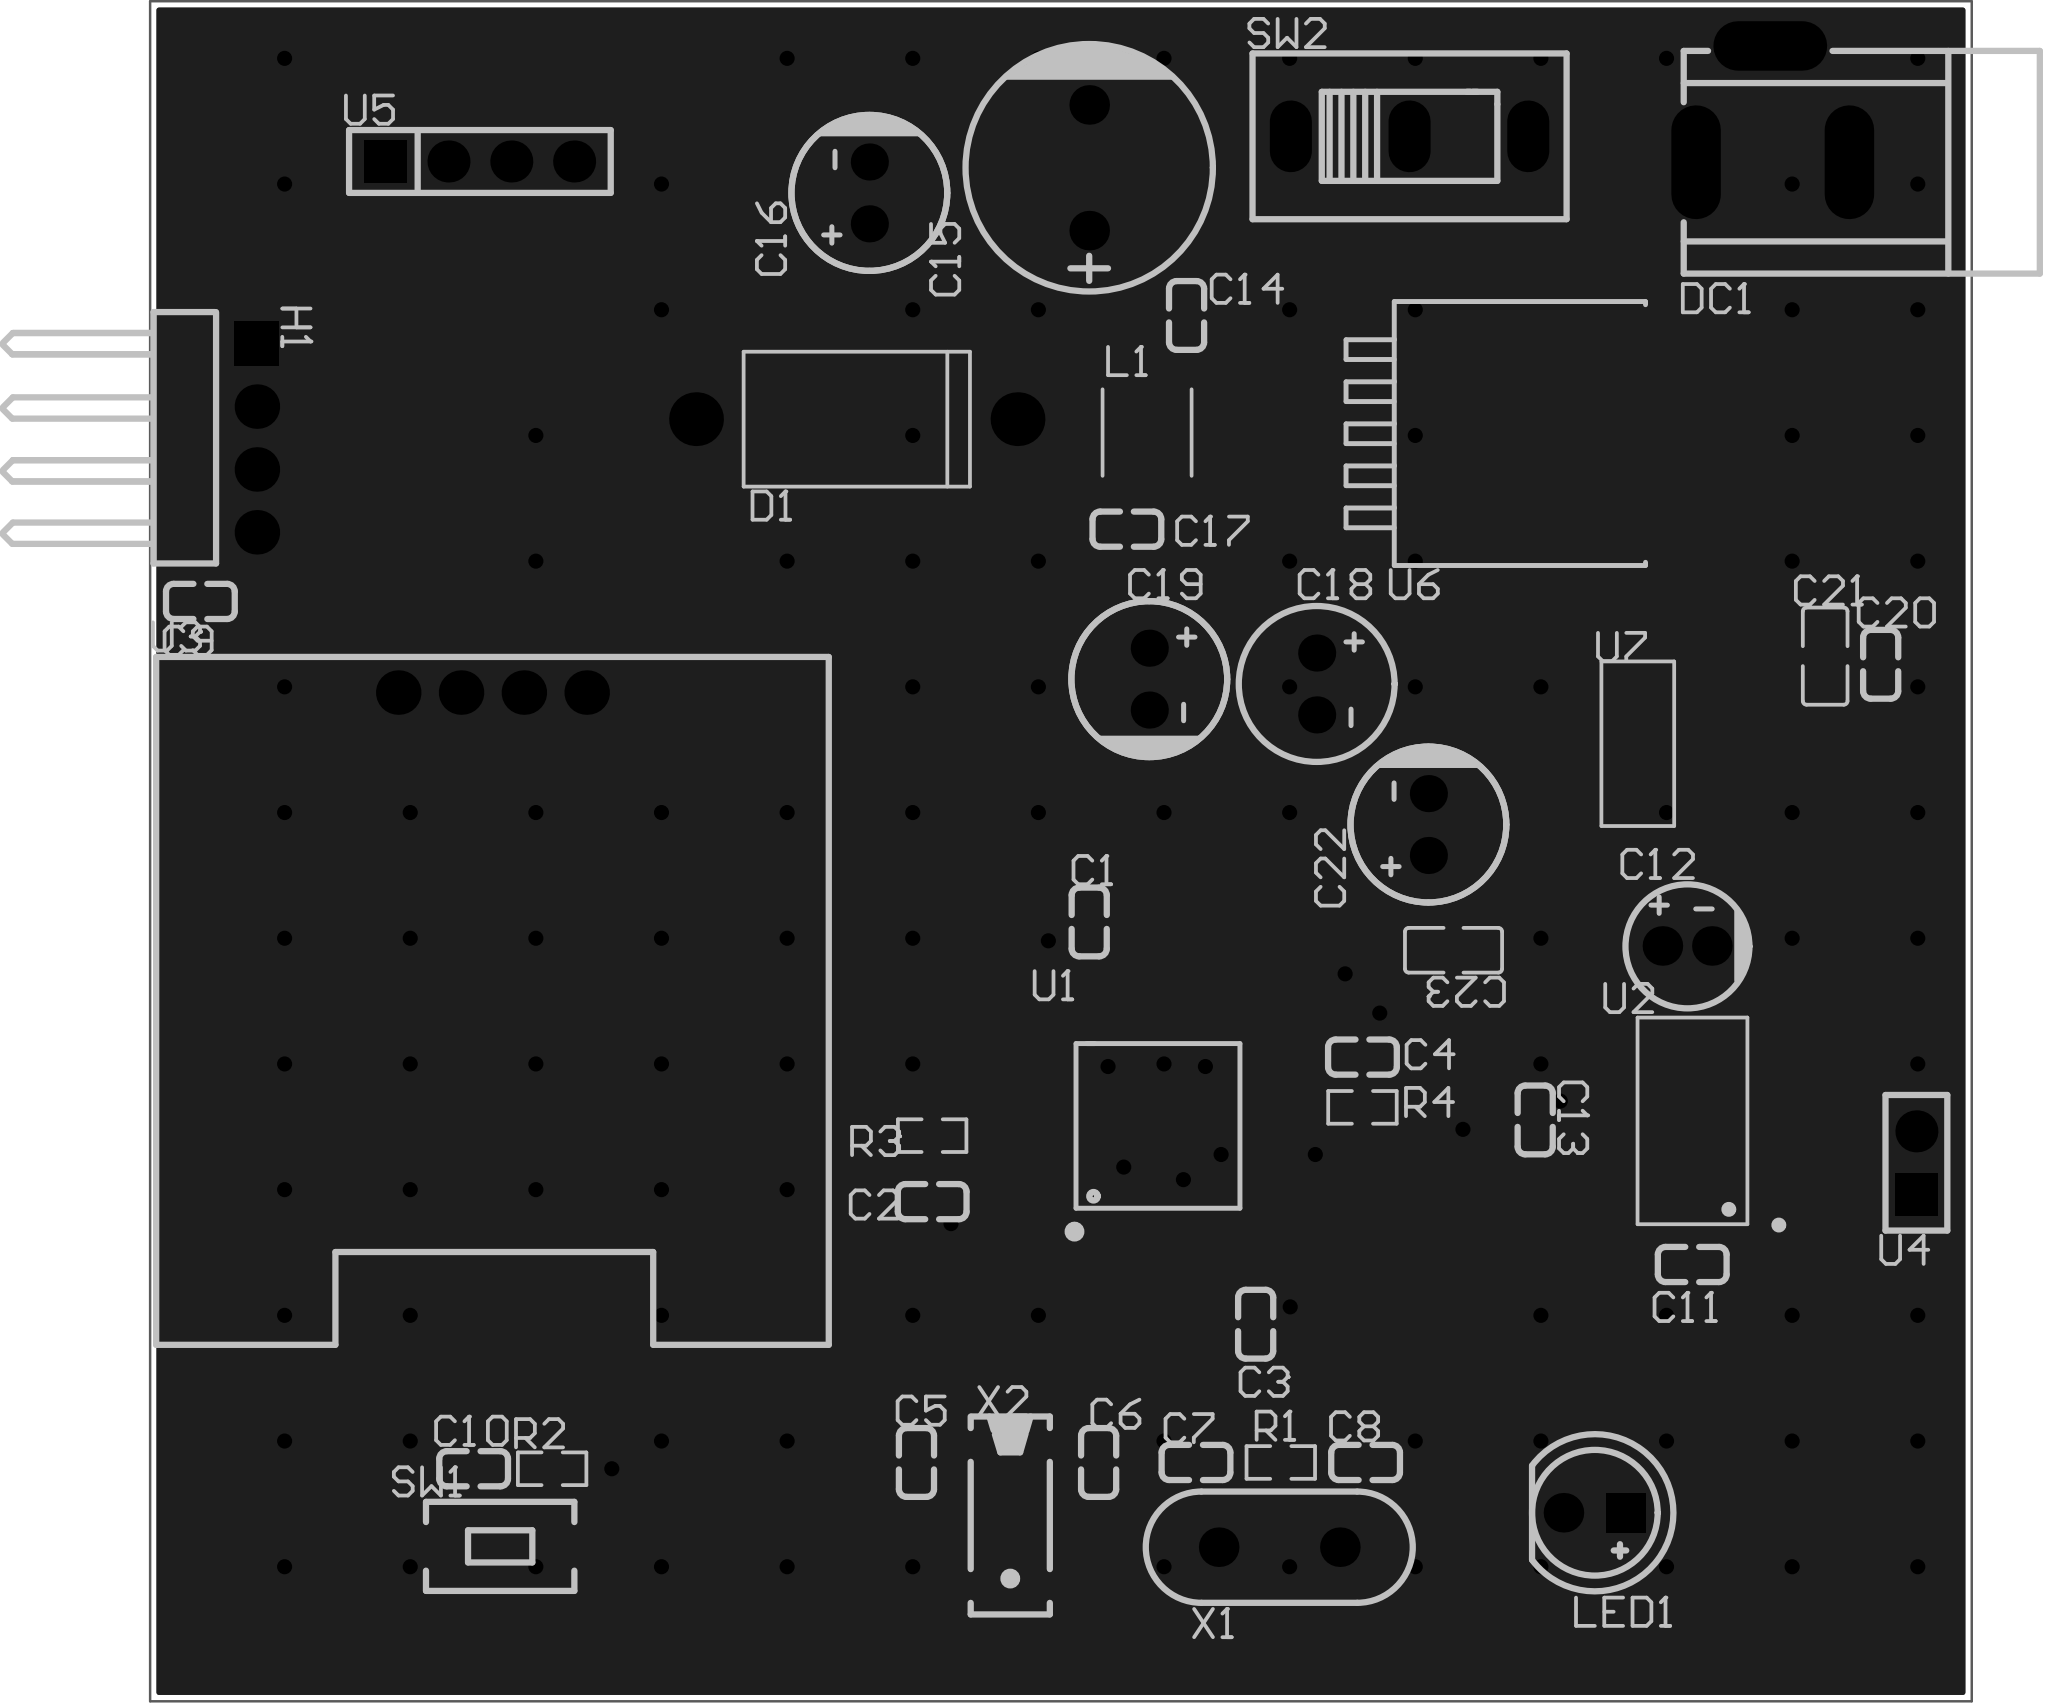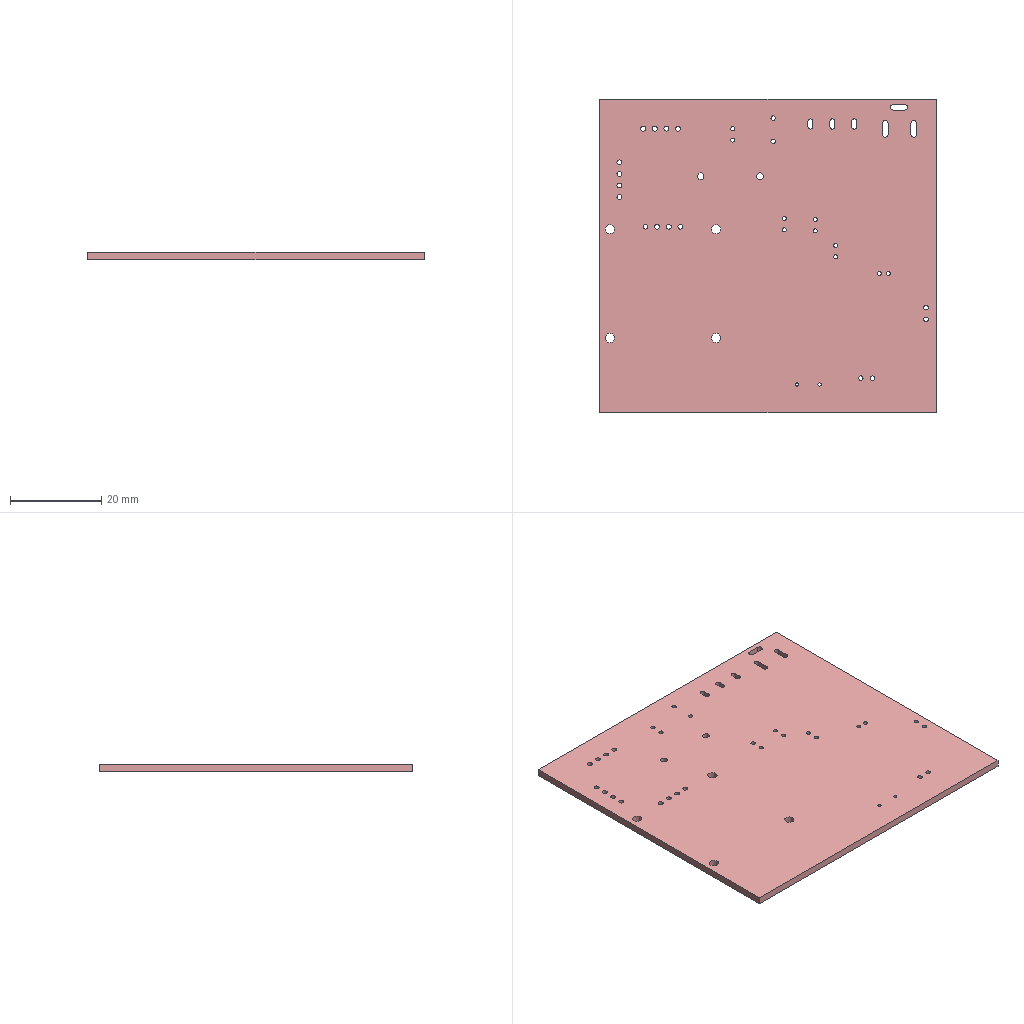Circuit board layout | Altium Designer | box 73.7 x 68.7 x 1.6 mm
Layer stack:
# Altium Designer layer stack of  (unit mm; dielectric type: 0 none, 1 core, 2 prepreg, 3 surface material)
index,name,kind,layer,copper_thickness_mm,dielectric_type,dielectric_thickness_mm,dielectric_material,dielectric_constant
0,Top Paste Mask Layer,other,,,,,,
1,Top Silkscreen Layer,other,,,,,,
2,Top Solder Mask Layer,dielectric,,,3,0.01,,3.3
3,Top Layer,copper,Top Layer,0.035,,,,
4,Dielectric1,dielectric,,,3,1.51,FR4,4.5
5,Bottom Layer,copper,Bottom Layer,0.035,,,,
6,Bottom Solder Mask Layer,dielectric,,,3,0.01,,3.3
7,Bottom Silkscreen Layer,other,,,,,,
8,Bottom Paste Mask Layer,other,,,,,,
# drill layer pairs: low layer,high layer
drill_pair,Top Layer,Bottom Layer
Part placement:
Designator,Comment,Layer,Footprint,Center-X(mm),Center-Y(mm),Rotation
C1,100nF,TopLayer,C0603,124.587,124.333,270
C2,100nF,TopLayer,C0603,118.237,113.03,0
C3,100nF,TopLayer,C0603,131.318,108.077,90
C4,100nF,TopLayer,C0603,135.636,118.872,180
C5,20pF,TopLayer,C0603,117.602,102.489,270
C6,20pF,TopLayer,C0603,124.968,102.489,270
C7,20pF,TopLayer,C0603,128.905,102.489,180
C8,20pF,TopLayer,C0603,135.763,102.489,0
C9,100nF,TopLayer,C0603,88.646,137.287,180
C10,1uF,TopLayer,C0603,99.695,102.235,0
C11,100nF,TopLayer,C0603,148.971,110.49,180
C12,10uF,TopLayer,CAP-TH_BD5.0-P2.00-D0.5-FD-A,148.765,123.364,0
C13,100nF,TopLayer,C0603,142.621,116.332,270
C14,100nF,TopLayer,C0603,128.524,148.844,270
C15,220uF,TopLayer,CAP-TH_BD10.0-P5.00-D1.0-FD,124.587,154.813,90
C16,100uF,TopLayer,CAP-TH_BD6.3-P2.50-D0.5-FD,115.697,153.797,90
C17,100nF,TopLayer,C0603,126.111,140.208,0
C18,220uF,TopLayer,CAP-TH_BD6.3-P2.50-D0.5-FD_DXW025M227E112S1AA,133.785,133.951,270
C19,100uF,TopLayer,CAP-TH_BD6.3-P2.50-D0.5-FD,127.016,134.147,270
C20,100nF,TopLayer,C0603,156.591,134.747,270
C21,10uF,TopLayer,C0805,154.347,135.076,270
C22,100uF,TopLayer,CAP-TH_BD6.3-P2.50-D0.5-FD,138.303,128.27,90
C23,10uF,TopLayer,C0805,139.319,123.19,180
D1,1N5824,TopLayer,DO-201AD_BD5.3-L9.0-P13.00-D1.3-RD,115.189,144.653,180
DC1,DC005,TopLayer,DC-IN-TH_DC005,152.227,157.386,180
H1,PZ254R-11-04P,TopLayer,HDR-TH_4P-P2.54-H-M-W10.4,90.932,143.891,270
L1,33uH,TopLayer,IND-SMD_L3.5-W3.0,126.927,144.111,90
LED1,BL-BUB1V4V-AT,TopLayer,LED-TH_BD5.8-P2.54-FD_RED,145.034,100.457,180
R1,1MΩ,TopLayer,R0603,132.334,102.489,180
R2,10kΩ,TopLayer,R0603,102.87,102.235,0
R3,100kΩ,TopLayer,R0603,118.237,115.697,0
R4,100kΩ,TopLayer,R0603,135.636,116.84,180
SW1,TS-1101-C-W,TopLayer,SW-SMD_L6.0-W3.3-LS8.0_TS-1101-C-W,100.769,99.098,0
SW2,SS12D10G4,TopLayer,SW-TH_3P-P4.80-HX-SS12D10G4,137.541,156.083,0
U1,STM32F103C8T6,TopLayer,LQFP-48_L7.0-W7.0-P0.50-LS9.0-BL,127.381,116.078,0
U2,TB6612FNG,TopLayer,SSOP-24_L8.4-W5.8-P0.65-LS7.8-BL,148.981,116.293,90
U3,HS96L03W2C03,TopLayer,OLED-TH_L27.8-W27.2-P2.54_C9900033791,100.457,133.604,0
U4,2.54-1*2P母,TopLayer,HDR-TH_2P-P2.54-V-F,158.036,114.601,90
U5,2.54-1*4P母,TopLayer,HDR-TH_4P-P2.54-V-F,99.949,155.067,0
U6,LM2596SX-5.0-JSM,TopLayer,TO-263-5_L10.0-W8.4-P1.70-LS15.3-BR,138.173,144.073,180
U7,AMS1117-3.3,TopLayer,SOT-223-3_L6.5-W3.4-P2.30-LS7.0-BR,146.87,131.536,0
X1,8MHz,TopLayer,OSC-TH_L10.0-W4.5-P5.00,132.273,99.065,90
X2,32.768kHz,TopLayer,MC-306_4P-L8.0-W3.2-P5.5-BL,121.395,100.347,270
Pad and via stacks:
# Altium Designer via and pad stacks of  (unit mm). Each distinct definition once, with the count of objects using it.
# via: kind,start_layer,end_layer,hole_mm,diameter_mm,mode(0 simple;1 top-mid-bottom;2 full stack),diameter_per_layer,count,example_net
# pad: kind,layer,hole_mm,hole_type(0 round;1 square;2 slot),plating,top_size,top_shape(1 round;2 rect;3 octagon;9 rounded rect),mid_size,bottom_size,mode,footprint,size_per_layer,count,example
pad,Top Layer,0,0,plated,0.8x0.9,2,0.8x0.9,0.8x0.9,0,C0603,,30,C1.2
pad,Top Layer,0,0,plated,1.41x1.35,2,1.41x1.35,1.41x1.35,0,C0805,,4,C21.2
pad,Top Layer,0,0,plated,1.8x3.12,2,1.8x3.12,1.8x3.12,0,IND-SMD_L3.5-W3.0,,2,L1.1
pad,Top Layer,0,0,plated,0.8065x0.864,2,0.8065x0.864,0.8065x0.864,0,R0603,,8,R1.2
pad,Top Layer,0,0,plated,1.2x1,2,1.2x1,1.2x1,0,SW-SMD_L6.0-W3.3-LS8.0_TS-1101-C-W,,2,SW1.1
pad,Top Layer,0,0,plated,0.27x1.5,1,0.27x1.5,0.27x1.5,0,LQFP-48_L7.0-W7.0-P0.50-LS9.0-BL,,24,U1.1
pad,Top Layer,0,0,plated,1.5x0.27,1,1.5x0.27,1.5x0.27,0,LQFP-48_L7.0-W7.0-P0.50-LS9.0-BL,,24,U1.13
pad,Top Layer,0,0,plated,0.364x2.082,1,0.364x2.082,0.364x2.082,0,SSOP-24_L8.4-W5.8-P0.65-LS7.8-BL,,24,U2.1
pad,Top Layer,0,0,plated,4x1.02,2,4x1.02,4x1.02,0,TO-263-5_L10.0-W8.4-P1.70-LS15.3-BR,,5,U6.1
pad,Top Layer,0,0,plated,8.4x10,2,8.4x10,8.4x10,0,TO-263-5_L10.0-W8.4-P1.70-LS15.3-BR,,1,U6.6
pad,Top Layer,0,0,plated,2.5x1.1,2,2.5x1.1,2.5x1.1,0,SOT-223-3_L6.5-W3.4-P2.30-LS7.0-BR,,3,U7.1
pad,Top Layer,0,0,plated,2.34x3.6,2,2.34x3.6,2.34x3.6,0,SOT-223-3_L6.5-W3.4-P2.30-LS7.0-BR,,1,U7.4
pad,Top Layer,0,0,plated,0.9x1.3,2,0.9x1.3,0.9x1.3,0,MC-306_4P-L8.0-W3.2-P5.5-BL,,4,X2.1
pad,Multi-Layer,0.9,0,plated,1.6x1.6,1,1.6x1.6,1.6x1.6,0,CAP-TH_BD5.0-P2.00-D0.5-FD-A,,2,C12.2
pad,Multi-Layer,1,0,plated,1.6x1.6,1,1.6x1.6,1.6x1.6,0,CAP-TH_BD10.0-P5.00-D1.0-FD,,2,C15.1
pad,Multi-Layer,0.9,0,plated,1.5x1.5,1,1.5x1.5,1.5x1.5,0,CAP-TH_BD6.3-P2.50-D0.5-FD,,6,C16.2
pad,Multi-Layer,0.9,0,plated,1.5x1.5,1,1.5x1.5,1.5x1.5,0,CAP-TH_BD6.3-P2.50-D0.5-FD_DXW025M227E112S1AA,,2,C18.1
pad,Multi-Layer,1.45,0,plated,2.175x2.175,1,2.175x2.175,2.175x2.175,0,DO-201AD_BD5.3-L9.0-P13.00-D1.3-RD,,2,D1.1
pad,Multi-Layer,1.2,2,plated,2x4.6,1,2x4.6,2x4.6,0,DC-IN-TH_DC005,,2,DC1.1
pad,Multi-Layer,1.2,2,plated,4.6x2,1,4.6x2,4.6x2,0,DC-IN-TH_DC005,,1,DC1.3
pad,Multi-Layer,1.1,0,plated,1.8x1.8,2,1.8x1.8,1.8x1.8,0,HDR-TH_4P-P2.54-H-M-W10.4,,1,H1.1
pad,Multi-Layer,1.1,0,plated,1.8x1.8,1,1.8x1.8,1.8x1.8,0,HDR-TH_4P-P2.54-H-M-W10.4,,3,H1.2
pad,Multi-Layer,1,0,plated,1.6x1.6,1,1.6x1.6,1.6x1.6,0,LED-TH_BD5.8-P2.54-FD_RED,,1,LED1.2
pad,Multi-Layer,1,0,plated,1.6x1.6,2,1.6x1.6,1.6x1.6,0,LED-TH_BD5.8-P2.54-FD_RED,,1,LED1.1
pad,Multi-Layer,1.1,2,plated,1.7x2.9,1,1.7x2.9,1.7x2.9,0,SW-TH_3P-P4.80-HX-SS12D10G4,,3,SW2.1
pad,Multi-Layer,1.05,0,plated,1.8x1.8,1,1.8x1.8,1.8x1.8,0,OLED-TH_L27.8-W27.2-P2.54_C9900033791,,4,U3.1
pad,Multi-Layer,1,0,plated,1.7x1.7,2,1.7x1.7,1.7x1.7,0,HDR-TH_2P-P2.54-V-F,,1,U4.1
pad,Multi-Layer,1,0,plated,1.7x1.7,1,1.7x1.7,1.7x1.7,0,HDR-TH_2P-P2.54-V-F,,1,U4.2
pad,Multi-Layer,1.1,0,plated,1.7x1.7,2,1.7x1.7,1.7x1.7,0,HDR-TH_4P-P2.54-V-F,,1,U5.1
pad,Multi-Layer,1.1,0,plated,1.7x1.7,1,1.7x1.7,1.7x1.7,0,HDR-TH_4P-P2.54-V-F,,3,U5.2
pad,Multi-Layer,0.7,0,plated,1.6x1.6,1,1.6x1.6,1.6x1.6,0,OSC-TH_L10.0-W4.5-P5.00,,2,X1.2
via,Top Layer,Bottom Layer,0.3048,0.61,0,,122,PB4
Copper pours:
name,layer,net,type(0 solid;1 hatched;2 none)
Top Layer-GND,Top Layer,GND,0
Bottom Layer-GND,Bottom Layer,GND,0
Design rules, without the lines most boards share:
# Altium Designer design rules of  (exported by Altium Designer, unit mm)
# columns: name | kind | enabled | priority | scope1 | scope2 | descriptor | typed fields (field=value)
creepage | 65 | enabled | 1 | All | All | Creepage Distance Constraint =(0mil) (All),(All) |